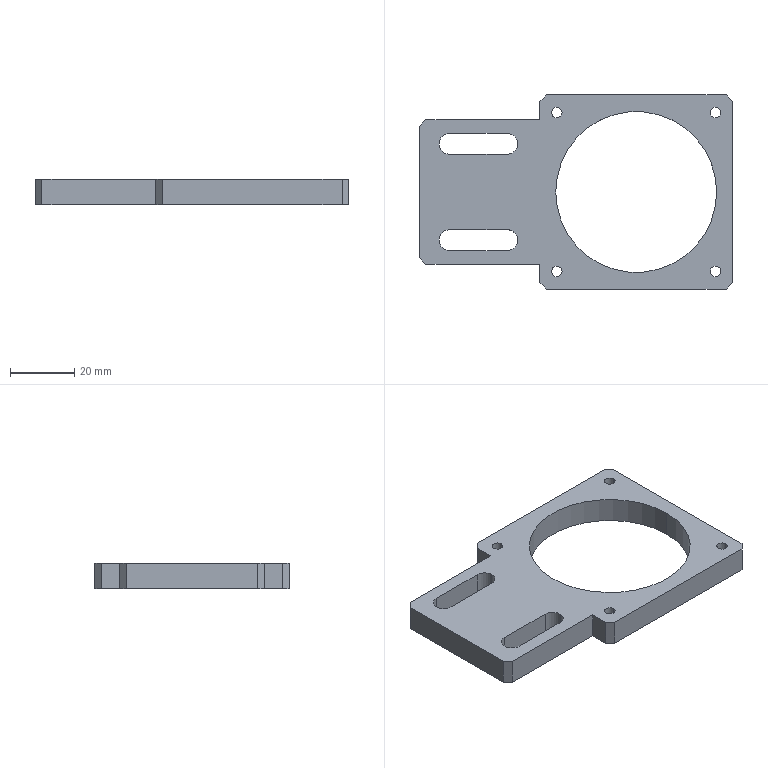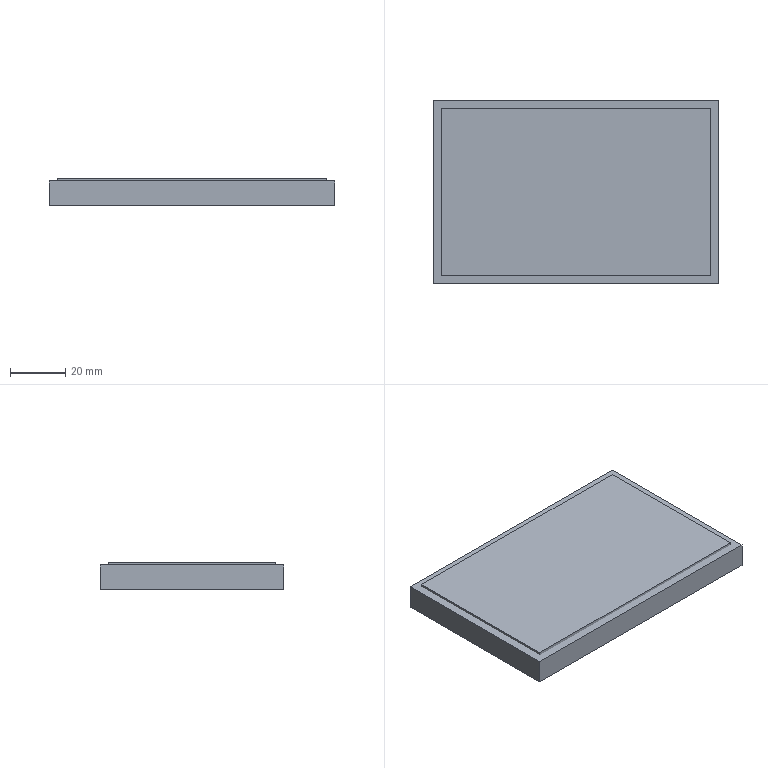CAM job | NX | 3-axis milling, drilling | part box 97.5 x 60.5 x 8 mm | stock box 103.5 x 66.5 x 10 mm
Tools:
number,name,description,diameter,corner_radius,flute_length,length,flutes
1,D63,Milling Tool-5 Parameters,63.0,0.0,50.0,75.0,2
7,D6A45,Milling Tool-5 Parameters,6.0,0.0,3.0,3.0,2
13,3.4ZT,Drilling Tool,3.3,0.0,35.0,50.0,2
12,M4,Milling Tool-5 Parameters,3.3,0.0,30.0,30.0,4
10,D10,Milling Tool-5 Parameters,10.0,0.0,50.0,75.0,2
4,D4,Milling Tool-5 Parameters,4.0,0.0,50.0,75.0,2
Operations:
program,operation,operation_type,tool,method,geometry_group,spindle_rpm,surface_speed,feed_per_tooth,feed_cut,feed_plunge,cut_length_mm,path_length_mm,cut_time_min,machine_time_min
1-101-65-10毛胚,FLOOR_WALL,VolumeBased25DMillingOperation,D63,METHOD,A,6500.0,1286.0,0.0962,1250.0,100.0,386.297,440.297,0.309,0.3144
1-101-65-10毛胚,DRILLING_COPY_1,Operation,D6A45,METHOD,A,3000.0,56.0,0.0333,200.0,0.0,25.5,292.433,0.1275,0.1542
1-101-65-10毛胚,DRILLING_COPY_1_COPY_COPY_COPY_COPY,Operation,3.4ZT,METHOD,A,2000.0,20.0,0.0375,150.0,0.0,49.966,317.696,0.3331,0.3599
1-101-65-10毛胚,DRILLING_COPY_1_COPY_COPY_COPY_COPY_1,Operation,M4,METHOD,A,200.0,2.0,0.0009,0.7,0.0,44.0,305.765,62.857,62.883
1-101-65-10毛胚,ADAPTIVE_MILLING,CavityMilling,D10,METHOD,A,7000.0,219.0,0.2143,3000.0,1000.0,5034.957,5217.154,2.1,2.119
1-101-65-10毛胚,ZLEVEL_PROFILE,ZLevelMilling,D4,METHOD,A,7000.0,87.0,0.0929,1300.0,1000.0,2472.814,2636.025,1.918,1.934
1-101-65-10毛胚,ZLEVEL_PROFILE_COPY_1,ZLevelMilling,D4,METHOD,A,7000.0,87.0,0.1071,1500.0,1000.0,272.882,590.588,0.1938,0.2255
1-101-65-10毛胚,ZLEVEL_PROFILE_COPY_COPY_1,ZLevelMilling,D4,METHOD,A,7000.0,219.0,0.0714,1000.0,100.0,474.509,657.264,0.4745,0.4928
1-101-65-10毛胚,ZLEVEL_PROFILE_COPY_1_COPY_COPY_COPY_COPY_2_COPY,ZLevelMilling,D6A45,METHOD,A,7000.0,131.0,0.0714,1000.0,1000.0,603.241,1438.68,0.6032,0.6868
1-101-65-10毛胚,刀补11,ZLevelMilling,D4,METHOD,A,7000.0,219.0,0.0714,1000.0,100.0,114.227,333.157,0.1142,0.1361
2-101-65-10毛胚,FLOOR_WALL_COPY,VolumeBased25DMillingOperation,D63,METHOD,B,6500.0,1286.0,0.0962,1250.0,100.0,736.594,877.891,0.5893,0.6034
2-101-65-10毛胚,ZLEVEL_PROFILE_COPY_1_COPY_COPY_COPY_COPY_2_COPY_COPY,ZLevelMilling,D6A45,METHOD,B,7000.0,131.0,0.0714,1000.0,1000.0,603.241,1467.471,0.6032,0.6897